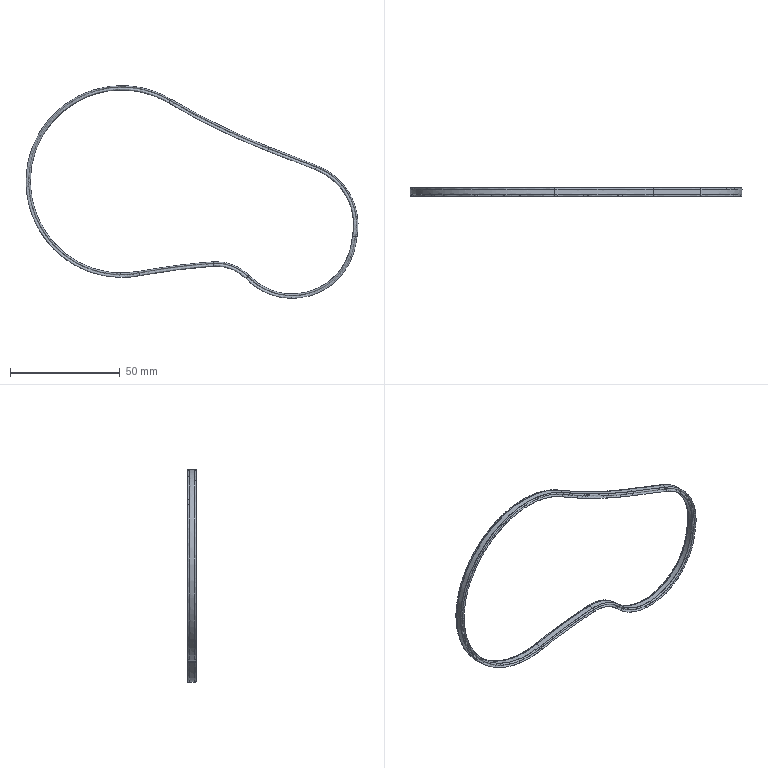Part | SolidWorks | features BaseBody 1 | 1 solid | 56 faces | box 151.361 x 3.9 x 96.963 mm | volume 2710 mm3 | spline 54 | plane 2